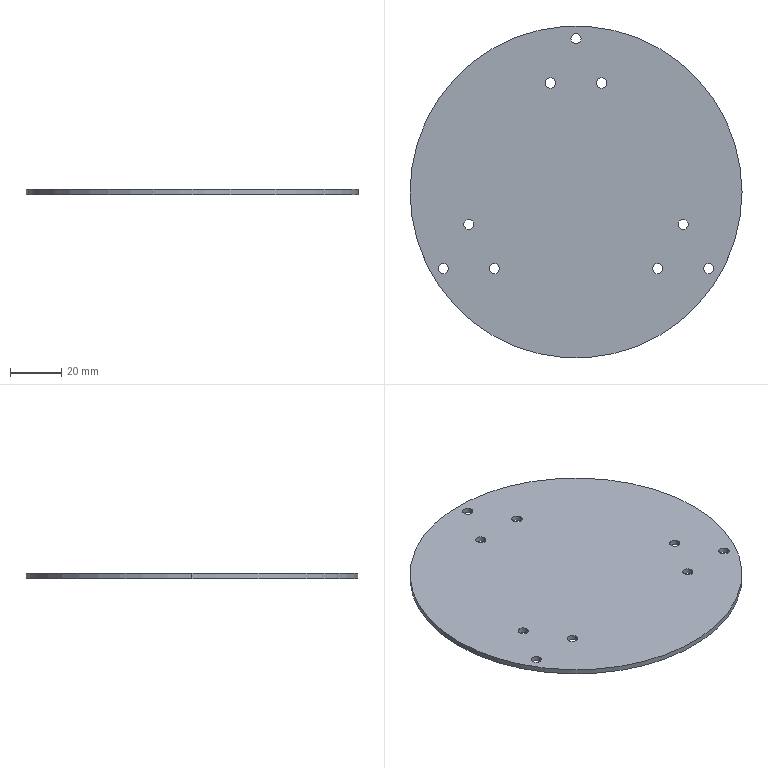Part | SolidWorks | features Extrusion 1, ICE 1 | 1 solid | 22 faces | box 130 x 130 x 2 mm | volume 26320 mm3 | cylinder 20 | plane 2 | commonest cylinder face diameters 4 x18 130 x2
STEP:
#1=CARTESIAN_POINT('',(-33.962,-30.,0.));
#2=VERTEX_POINT('',#1);
#3=CARTESIAN_POINT('',(-29.962,-30.,0.));
#4=VERTEX_POINT('',#3);
#5=CARTESIAN_POINT('',(-31.962,-30.,0.));
#6=DIRECTION('',(0.,0.,1.));
#7=DIRECTION('',(1.,0.,0.));
#8=AXIS2_PLACEMENT_3D('',#5,#6,#7);
#9=CIRCLE('',#8,2.);
#10=EDGE_CURVE('',#2,#4,#9,.T.);
#11=ORIENTED_EDGE('',*,*,#10,.F.);
#12=CARTESIAN_POINT('',(-33.962,-30.,2.));
#13=VERTEX_POINT('',#12);
#14=CARTESIAN_POINT('',(-33.962,-30.,0.));
#15=DIRECTION('',(0.,0.,1.));
#16=VECTOR('',#15,1000.);
#17=LINE('',#14,#16);
#18=EDGE_CURVE('',#2,#13,#17,.T.);
#19=ORIENTED_EDGE('',*,*,#18,.T.);
#20=CARTESIAN_POINT('',(-29.962,-30.,2.));
#21=VERTEX_POINT('',#20);
#22=CARTESIAN_POINT('',(-31.962,-30.,2.));
#23=DIRECTION('',(0.,0.,1.));
#24=DIRECTION('',(1.,0.,0.));
#25=AXIS2_PLACEMENT_3D('',#22,#23,#24);
#26=CIRCLE('',#25,2.);
#27=EDGE_CURVE('',#13,#21,#26,.T.);
#28=ORIENTED_EDGE('',*,*,#27,.T.);
#29=CARTESIAN_POINT('',(-29.962,-30.,0.));
#30=DIRECTION('',(0.,0.,1.));
#31=VECTOR('',#30,1000.);
#32=LINE('',#29,#31);
#33=EDGE_CURVE('',#4,#21,#32,.T.);
#34=ORIENTED_EDGE('',*,*,#33,.F.);
#35=EDGE_LOOP('',(#11,#19,#28,#34));
#36=FACE_OUTER_BOUND('',#35,.T.);
#37=CARTESIAN_POINT('',(-31.962,-30.,0.));
#38=DIRECTION('',(0.,0.,1.));
#39=DIRECTION('',(1.,0.,0.));
#40=AXIS2_PLACEMENT_3D('',#37,#38,#39);
#41=CYLINDRICAL_SURFACE('',#40,2.);
#42=ADVANCED_FACE('',(#36),#41,.F.);
#43=CARTESIAN_POINT('',(-43.962,-12.679,0.));
#44=VERTEX_POINT('',#43);
#45=CARTESIAN_POINT('',(-39.962,-12.679,0.));
#46=VERTEX_POINT('',#45);
#47=CARTESIAN_POINT('',(-41.962,-12.679,0.));
#48=DIRECTION('',(0.,0.,1.));
#49=DIRECTION('',(1.,0.,0.));
#50=AXIS2_PLACEMENT_3D('',#47,#48,#49);
#51=CIRCLE('',#50,2.);
#52=EDGE_CURVE('',#44,#46,#51,.T.);
#53=ORIENTED_EDGE('',*,*,#52,.F.);
#54=CARTESIAN_POINT('',(-43.962,-12.679,2.));
#55=VERTEX_POINT('',#54);
#56=CARTESIAN_POINT('',(-43.962,-12.679,0.));
#57=DIRECTION('',(0.,0.,1.));
#58=VECTOR('',#57,1000.);
#59=LINE('',#56,#58);
#60=EDGE_CURVE('',#44,#55,#59,.T.);
#61=ORIENTED_EDGE('',*,*,#60,.T.);
#62=CARTESIAN_POINT('',(-39.962,-12.679,2.));
#63=VERTEX_POINT('',#62);
#64=CARTESIAN_POINT('',(-41.962,-12.679,2.));
#65=DIRECTION('',(0.,0.,1.));
#66=DIRECTION('',(1.,0.,0.));
#67=AXIS2_PLACEMENT_3D('',#64,#65,#66);
#68=CIRCLE('',#67,2.);
#69=EDGE_CURVE('',#55,#63,#68,.T.);
#70=ORIENTED_EDGE('',*,*,#69,.T.);
#71=CARTESIAN_POINT('',(-39.962,-12.679,0.));
#72=DIRECTION('',(0.,0.,1.));
#73=VECTOR('',#72,1000.);
#74=LINE('',#71,#73);
#75=EDGE_CURVE('',#46,#63,#74,.T.);
#76=ORIENTED_EDGE('',*,*,#75,.F.);
#77=EDGE_LOOP('',(#53,#61,#70,#76));
#78=FACE_OUTER_BOUND('',#77,.T.);
#79=CARTESIAN_POINT('',(-41.962,-12.679,0.));
#80=DIRECTION('',(0.,0.,1.));
#81=DIRECTION('',(1.,0.,0.));
#82=AXIS2_PLACEMENT_3D('',#79,#80,#81);
#83=CYLINDRICAL_SURFACE('',#82,2.);
#84=ADVANCED_FACE('',(#78),#83,.F.);
#85=CARTESIAN_POINT('',(-53.962,-30.,0.));
#86=VERTEX_POINT('',#85);
#87=CARTESIAN_POINT('',(-49.962,-30.,0.));
#88=VERTEX_POINT('',#87);
#89=CARTESIAN_POINT('',(-51.962,-30.,0.));
#90=DIRECTION('',(0.,0.,1.));
#91=DIRECTION('',(1.,0.,0.));
#92=AXIS2_PLACEMENT_3D('',#89,#90,#91);
#93=CIRCLE('',#92,2.);
#94=EDGE_CURVE('',#86,#88,#93,.T.);
#95=ORIENTED_EDGE('',*,*,#94,.F.);
#96=CARTESIAN_POINT('',(-53.962,-30.,2.));
#97=VERTEX_POINT('',#96);
#98=CARTESIAN_POINT('',(-53.962,-30.,0.));
#99=DIRECTION('',(0.,0.,1.));
#100=VECTOR('',#99,1000.);
#101=LINE('',#98,#100);
#102=EDGE_CURVE('',#86,#97,#101,.T.);
#103=ORIENTED_EDGE('',*,*,#102,.T.);
#104=CARTESIAN_POINT('',(-49.962,-30.,2.));
#105=VERTEX_POINT('',#104);
#106=CARTESIAN_POINT('',(-51.962,-30.,2.));
#107=DIRECTION('',(0.,0.,1.));
#108=DIRECTION('',(1.,0.,0.));
#109=AXIS2_PLACEMENT_3D('',#106,#107,#108);
#110=CIRCLE('',#109,2.);
#111=EDGE_CURVE('',#97,#105,#110,.T.);
#112=ORIENTED_EDGE('',*,*,#111,.T.);
#113=CARTESIAN_POINT('',(-49.962,-30.,0.));
#114=DIRECTION('',(0.,0.,1.));
#115=VECTOR('',#114,1000.);
#116=LINE('',#113,#115);
#117=EDGE_CURVE('',#88,#105,#116,.T.);
#118=ORIENTED_EDGE('',*,*,#117,.F.);
#119=EDGE_LOOP('',(#95,#103,#112,#118));
#120=FACE_OUTER_BOUND('',#119,.T.);
#121=CARTESIAN_POINT('',(-51.962,-30.,0.));
#122=DIRECTION('',(0.,0.,1.));
#123=DIRECTION('',(1.,0.,0.));
#124=AXIS2_PLACEMENT_3D('',#121,#122,#123);
#125=CYLINDRICAL_SURFACE('',#124,2.);
#126=ADVANCED_FACE('',(#120),#125,.F.);
#127=CARTESIAN_POINT('',(39.962,-12.679,0.));
#128=VERTEX_POINT('',#127);
#129=CARTESIAN_POINT('',(43.962,-12.679,0.));
#130=VERTEX_POINT('',#129);
#131=CARTESIAN_POINT('',(41.962,-12.679,0.));
#132=DIRECTION('',(0.,0.,1.));
#133=DIRECTION('',(1.,0.,0.));
#134=AXIS2_PLACEMENT_3D('',#131,#132,#133);
#135=CIRCLE('',#134,2.);
#136=EDGE_CURVE('',#128,#130,#135,.T.);
#137=ORIENTED_EDGE('',*,*,#136,.F.);
#138=CARTESIAN_POINT('',(39.962,-12.679,2.));
#139=VERTEX_POINT('',#138);
#140=CARTESIAN_POINT('',(39.962,-12.679,0.));
#141=DIRECTION('',(0.,0.,1.));
#142=VECTOR('',#141,1000.);
#143=LINE('',#140,#142);
#144=EDGE_CURVE('',#128,#139,#143,.T.);
#145=ORIENTED_EDGE('',*,*,#144,.T.);
#146=CARTESIAN_POINT('',(43.962,-12.679,2.));
#147=VERTEX_POINT('',#146);
#148=CARTESIAN_POINT('',(41.962,-12.679,2.));
#149=DIRECTION('',(0.,0.,1.));
#150=DIRECTION('',(1.,0.,0.));
#151=AXIS2_PLACEMENT_3D('',#148,#149,#150);
#152=CIRCLE('',#151,2.);
#153=EDGE_CURVE('',#139,#147,#152,.T.);
#154=ORIENTED_EDGE('',*,*,#153,.T.);
#155=CARTESIAN_POINT('',(43.962,-12.679,0.));
#156=DIRECTION('',(0.,0.,1.));
#157=VECTOR('',#156,1000.);
#158=LINE('',#155,#157);
#159=EDGE_CURVE('',#130,#147,#158,.T.);
#160=ORIENTED_EDGE('',*,*,#159,.F.);
#161=EDGE_LOOP('',(#137,#145,#154,#160));
#162=FACE_OUTER_BOUND('',#161,.T.);
#163=CARTESIAN_POINT('',(41.962,-12.679,0.));
#164=DIRECTION('',(0.,0.,1.));
#165=DIRECTION('',(1.,0.,0.));
#166=AXIS2_PLACEMENT_3D('',#163,#164,#165);
#167=CYLINDRICAL_SURFACE('',#166,2.);
#168=ADVANCED_FACE('',(#162),#167,.F.);
#169=CARTESIAN_POINT('',(29.962,-30.,0.));
#170=VERTEX_POINT('',#169);
#171=CARTESIAN_POINT('',(33.962,-30.,0.));
#172=VERTEX_POINT('',#171);
#173=CARTESIAN_POINT('',(31.962,-30.,0.));
#174=DIRECTION('',(0.,0.,1.));
#175=DIRECTION('',(1.,0.,0.));
#176=AXIS2_PLACEMENT_3D('',#173,#174,#175);
#177=CIRCLE('',#176,2.);
#178=EDGE_CURVE('',#170,#172,#177,.T.);
#179=ORIENTED_EDGE('',*,*,#178,.F.);
#180=CARTESIAN_POINT('',(29.962,-30.,2.));
#181=VERTEX_POINT('',#180);
#182=CARTESIAN_POINT('',(29.962,-30.,0.));
#183=DIRECTION('',(0.,0.,1.));
#184=VECTOR('',#183,1000.);
#185=LINE('',#182,#184);
#186=EDGE_CURVE('',#170,#181,#185,.T.);
#187=ORIENTED_EDGE('',*,*,#186,.T.);
#188=CARTESIAN_POINT('',(33.962,-30.,2.));
#189=VERTEX_POINT('',#188);
#190=CARTESIAN_POINT('',(31.962,-30.,2.));
#191=DIRECTION('',(0.,0.,1.));
#192=DIRECTION('',(1.,0.,0.));
#193=AXIS2_PLACEMENT_3D('',#190,#191,#192);
#194=CIRCLE('',#193,2.);
#195=EDGE_CURVE('',#181,#189,#194,.T.);
#196=ORIENTED_EDGE('',*,*,#195,.T.);
#197=CARTESIAN_POINT('',(33.962,-30.,0.));
#198=DIRECTION('',(0.,0.,1.));
#199=VECTOR('',#198,1000.);
#200=LINE('',#197,#199);
#201=EDGE_CURVE('',#172,#189,#200,.T.);
#202=ORIENTED_EDGE('',*,*,#201,.F.);
#203=EDGE_LOOP('',(#179,#187,#196,#202));
#204=FACE_OUTER_BOUND('',#203,.T.);
#205=CARTESIAN_POINT('',(31.962,-30.,0.));
#206=DIRECTION('',(0.,0.,1.));
#207=DIRECTION('',(1.,0.,0.));
#208=AXIS2_PLACEMENT_3D('',#205,#206,#207);
#209=CYLINDRICAL_SURFACE('',#208,2.);
#210=ADVANCED_FACE('',(#204),#209,.F.);
#211=CARTESIAN_POINT('',(49.962,-30.,0.));
#212=VERTEX_POINT('',#211);
#213=CARTESIAN_POINT('',(53.962,-30.,0.));
#214=VERTEX_POINT('',#213);
#215=CARTESIAN_POINT('',(51.962,-30.,0.));
#216=DIRECTION('',(0.,0.,1.));
#217=DIRECTION('',(1.,0.,0.));
#218=AXIS2_PLACEMENT_3D('',#215,#216,#217);
#219=CIRCLE('',#218,2.);
#220=EDGE_CURVE('',#212,#214,#219,.T.);
#221=ORIENTED_EDGE('',*,*,#220,.F.);
#222=CARTESIAN_POINT('',(49.962,-30.,2.));
#223=VERTEX_POINT('',#222);
#224=CARTESIAN_POINT('',(49.962,-30.,0.));
#225=DIRECTION('',(0.,0.,1.));
#226=VECTOR('',#225,1000.);
#227=LINE('',#224,#226);
#228=EDGE_CURVE('',#212,#223,#227,.T.);
#229=ORIENTED_EDGE('',*,*,#228,.T.);
#230=CARTESIAN_POINT('',(53.962,-30.,2.));
#231=VERTEX_POINT('',#230);
#232=CARTESIAN_POINT('',(51.962,-30.,2.));
#233=DIRECTION('',(0.,0.,1.));
#234=DIRECTION('',(1.,0.,0.));
#235=AXIS2_PLACEMENT_3D('',#232,#233,#234);
#236=CIRCLE('',#235,2.);
#237=EDGE_CURVE('',#223,#231,#236,.T.);
#238=ORIENTED_EDGE('',*,*,#237,.T.);
#239=CARTESIAN_POINT('',(53.962,-30.,0.));
#240=DIRECTION('',(0.,0.,1.));
#241=VECTOR('',#240,1000.);
#242=LINE('',#239,#241);
#243=EDGE_CURVE('',#214,#231,#242,.T.);
#244=ORIENTED_EDGE('',*,*,#243,.F.);
#245=EDGE_LOOP('',(#221,#229,#238,#244));
#246=FACE_OUTER_BOUND('',#245,.T.);
#247=CARTESIAN_POINT('',(51.962,-30.,0.));
#248=DIRECTION('',(0.,0.,1.));
#249=DIRECTION('',(1.,0.,0.));
#250=AXIS2_PLACEMENT_3D('',#247,#248,#249);
#251=CYLINDRICAL_SURFACE('',#250,2.);
#252=ADVANCED_FACE('',(#246),#251,.F.);
#253=CARTESIAN_POINT('',(-12.,42.679,0.));
#254=VERTEX_POINT('',#253);
#255=CARTESIAN_POINT('',(-8.,42.679,0.));
#256=VERTEX_POINT('',#255);
#257=CARTESIAN_POINT('',(-10.,42.679,0.));
#258=DIRECTION('',(0.,0.,1.));
#259=DIRECTION('',(1.,0.,0.));
#260=AXIS2_PLACEMENT_3D('',#257,#258,#259);
#261=CIRCLE('',#260,2.);
#262=EDGE_CURVE('',#254,#256,#261,.T.);
#263=ORIENTED_EDGE('',*,*,#262,.F.);
#264=CARTESIAN_POINT('',(-12.,42.679,2.));
#265=VERTEX_POINT('',#264);
#266=CARTESIAN_POINT('',(-12.,42.679,0.));
#267=DIRECTION('',(0.,0.,1.));
#268=VECTOR('',#267,1000.);
#269=LINE('',#266,#268);
#270=EDGE_CURVE('',#254,#265,#269,.T.);
#271=ORIENTED_EDGE('',*,*,#270,.T.);
#272=CARTESIAN_POINT('',(-8.,42.679,2.));
#273=VERTEX_POINT('',#272);
#274=CARTESIAN_POINT('',(-10.,42.679,2.));
#275=DIRECTION('',(0.,0.,1.));
#276=DIRECTION('',(1.,0.,0.));
#277=AXIS2_PLACEMENT_3D('',#274,#275,#276);
#278=CIRCLE('',#277,2.);
#279=EDGE_CURVE('',#265,#273,#278,.T.);
#280=ORIENTED_EDGE('',*,*,#279,.T.);
#281=CARTESIAN_POINT('',(-8.,42.679,0.));
#282=DIRECTION('',(0.,0.,1.));
#283=VECTOR('',#282,1000.);
#284=LINE('',#281,#283);
#285=EDGE_CURVE('',#256,#273,#284,.T.);
#286=ORIENTED_EDGE('',*,*,#285,.F.);
#287=EDGE_LOOP('',(#263,#271,#280,#286));
#288=FACE_OUTER_BOUND('',#287,.T.);
#289=CARTESIAN_POINT('',(-10.,42.679,0.));
#290=DIRECTION('',(0.,0.,1.));
#291=DIRECTION('',(1.,0.,0.));
#292=AXIS2_PLACEMENT_3D('',#289,#290,#291);
#293=CYLINDRICAL_SURFACE('',#292,2.);
#294=ADVANCED_FACE('',(#288),#293,.F.);
#295=CARTESIAN_POINT('',(8.,42.679,0.));
#296=VERTEX_POINT('',#295);
#297=CARTESIAN_POINT('',(12.,42.679,0.));
#298=VERTEX_POINT('',#297);
#299=CARTESIAN_POINT('',(10.,42.679,0.));
#300=DIRECTION('',(0.,0.,1.));
#301=DIRECTION('',(1.,0.,0.));
#302=AXIS2_PLACEMENT_3D('',#299,#300,#301);
#303=CIRCLE('',#302,2.);
#304=EDGE_CURVE('',#296,#298,#303,.T.);
#305=ORIENTED_EDGE('',*,*,#304,.F.);
#306=CARTESIAN_POINT('',(8.,42.679,2.));
#307=VERTEX_POINT('',#306);
#308=CARTESIAN_POINT('',(8.,42.679,0.));
#309=DIRECTION('',(0.,0.,1.));
#310=VECTOR('',#309,1000.);
#311=LINE('',#308,#310);
#312=EDGE_CURVE('',#296,#307,#311,.T.);
#313=ORIENTED_EDGE('',*,*,#312,.T.);
#314=CARTESIAN_POINT('',(12.,42.679,2.));
#315=VERTEX_POINT('',#314);
#316=CARTESIAN_POINT('',(10.,42.679,2.));
#317=DIRECTION('',(0.,0.,1.));
#318=DIRECTION('',(1.,0.,0.));
#319=AXIS2_PLACEMENT_3D('',#316,#317,#318);
#320=CIRCLE('',#319,2.);
#321=EDGE_CURVE('',#307,#315,#320,.T.);
#322=ORIENTED_EDGE('',*,*,#321,.T.);
#323=CARTESIAN_POINT('',(12.,42.679,0.));
#324=DIRECTION('',(0.,0.,1.));
#325=VECTOR('',#324,1000.);
#326=LINE('',#323,#325);
#327=EDGE_CURVE('',#298,#315,#326,.T.);
#328=ORIENTED_EDGE('',*,*,#327,.F.);
#329=EDGE_LOOP('',(#305,#313,#322,#328));
#330=FACE_OUTER_BOUND('',#329,.T.);
#331=CARTESIAN_POINT('',(10.,42.679,0.));
#332=DIRECTION('',(0.,0.,1.));
#333=DIRECTION('',(1.,0.,0.));
#334=AXIS2_PLACEMENT_3D('',#331,#332,#333);
#335=CYLINDRICAL_SURFACE('',#334,2.);
#336=ADVANCED_FACE('',(#330),#335,.F.);
#337=CARTESIAN_POINT('',(-2.,60.,0.));
#338=VERTEX_POINT('',#337);
#339=CARTESIAN_POINT('',(2.,60.,0.));
#340=VERTEX_POINT('',#339);
#341=CARTESIAN_POINT('',(0.,60.,0.));
#342=DIRECTION('',(0.,0.,1.));
#343=DIRECTION('',(1.,0.,0.));
#344=AXIS2_PLACEMENT_3D('',#341,#342,#343);
#345=CIRCLE('',#344,2.);
#346=EDGE_CURVE('',#338,#340,#345,.T.);
#347=ORIENTED_EDGE('',*,*,#346,.F.);
#348=CARTESIAN_POINT('',(-2.,60.,2.));
#349=VERTEX_POINT('',#348);
#350=CARTESIAN_POINT('',(-2.,60.,0.));
#351=DIRECTION('',(0.,0.,1.));
#352=VECTOR('',#351,1000.);
#353=LINE('',#350,#352);
#354=EDGE_CURVE('',#338,#349,#353,.T.);
#355=ORIENTED_EDGE('',*,*,#354,.T.);
#356=CARTESIAN_POINT('',(2.,60.,2.));
#357=VERTEX_POINT('',#356);
#358=CARTESIAN_POINT('',(0.,60.,2.));
#359=DIRECTION('',(0.,0.,1.));
#360=DIRECTION('',(1.,0.,0.));
#361=AXIS2_PLACEMENT_3D('',#358,#359,#360);
#362=CIRCLE('',#361,2.);
#363=EDGE_CURVE('',#349,#357,#362,.T.);
#364=ORIENTED_EDGE('',*,*,#363,.T.);
#365=CARTESIAN_POINT('',(2.,60.,0.));
#366=DIRECTION('',(0.,0.,1.));
#367=VECTOR('',#366,1000.);
#368=LINE('',#365,#367);
#369=EDGE_CURVE('',#340,#357,#368,.T.);
#370=ORIENTED_EDGE('',*,*,#369,.F.);
#371=EDGE_LOOP('',(#347,#355,#364,#370));
#372=FACE_OUTER_BOUND('',#371,.T.);
#373=CARTESIAN_POINT('',(0.,60.,0.));
#374=DIRECTION('',(0.,0.,1.));
#375=DIRECTION('',(1.,0.,0.));
#376=AXIS2_PLACEMENT_3D('',#373,#374,#375);
#377=CYLINDRICAL_SURFACE('',#376,2.);
#378=ADVANCED_FACE('',(#372),#377,.F.);
#379=CARTESIAN_POINT('',(65.,0.,2.));
#380=VERTEX_POINT('',#379);
#381=CARTESIAN_POINT('',(-65.,0.,2.));
#382=VERTEX_POINT('',#381);
#383=CARTESIAN_POINT('',(0.,0.,2.));
#384=DIRECTION('',(0.,0.,1.));
#385=DIRECTION('',(1.,0.,0.));
#386=AXIS2_PLACEMENT_3D('',#383,#384,#385);
#387=CIRCLE('',#386,65.);
#388=EDGE_CURVE('',#380,#382,#387,.T.);
#389=ORIENTED_EDGE('',*,*,#388,.F.);
#390=CARTESIAN_POINT('',(65.,0.,0.));
#391=VERTEX_POINT('',#390);
#392=CARTESIAN_POINT('',(65.,0.,2.));
#393=DIRECTION('',(0.,0.,-1.));
#394=VECTOR('',#393,1000.);
#395=LINE('',#392,#394);
#396=EDGE_CURVE('',#380,#391,#395,.T.);
#397=ORIENTED_EDGE('',*,*,#396,.T.);
#398=CARTESIAN_POINT('',(-65.,0.,0.));
#399=VERTEX_POINT('',#398);
#400=CARTESIAN_POINT('',(0.,0.,0.));
#401=DIRECTION('',(0.,0.,1.));
#402=DIRECTION('',(1.,0.,0.));
#403=AXIS2_PLACEMENT_3D('',#400,#401,#402);
#404=CIRCLE('',#403,65.);
#405=EDGE_CURVE('',#391,#399,#404,.T.);
#406=ORIENTED_EDGE('',*,*,#405,.T.);
#407=CARTESIAN_POINT('',(-65.,0.,2.));
#408=DIRECTION('',(0.,0.,-1.));
#409=VECTOR('',#408,1000.);
#410=LINE('',#407,#409);
#411=EDGE_CURVE('',#382,#399,#410,.T.);
#412=ORIENTED_EDGE('',*,*,#411,.F.);
#413=EDGE_LOOP('',(#389,#397,#406,#412));
#414=FACE_OUTER_BOUND('',#413,.T.);
#415=CARTESIAN_POINT('',(0.,0.,2.));
#416=DIRECTION('',(0.,0.,-1.));
#417=DIRECTION('',(-1.,0.,0.));
#418=AXIS2_PLACEMENT_3D('',#415,#416,#417);
#419=CYLINDRICAL_SURFACE('',#418,65.);
#420=ADVANCED_FACE('',(#414),#419,.T.);
#421=ORIENTED_EDGE('',*,*,#396,.F.);
#422=CARTESIAN_POINT('',(0.,0.,2.));
#423=DIRECTION('',(0.,0.,1.));
#424=DIRECTION('',(1.,0.,0.));
#425=AXIS2_PLACEMENT_3D('',#422,#423,#424);
#426=CIRCLE('',#425,65.);
#427=EDGE_CURVE('',#382,#380,#426,.T.);
#428=ORIENTED_EDGE('',*,*,#427,.F.);
#429=ORIENTED_EDGE('',*,*,#411,.T.);
#430=CARTESIAN_POINT('',(0.,0.,0.));
#431=DIRECTION('',(0.,0.,1.));
#432=DIRECTION('',(1.,0.,0.));
#433=AXIS2_PLACEMENT_3D('',#430,#431,#432);
#434=CIRCLE('',#433,65.);
#435=EDGE_CURVE('',#399,#391,#434,.T.);
#436=ORIENTED_EDGE('',*,*,#435,.T.);
#437=EDGE_LOOP('',(#421,#428,#429,#436));
#438=FACE_OUTER_BOUND('',#437,.T.);
#439=CARTESIAN_POINT('',(0.,0.,2.));
#440=DIRECTION('',(0.,0.,-1.));
#441=DIRECTION('',(-1.,0.,0.));
#442=AXIS2_PLACEMENT_3D('',#439,#440,#441);
#443=CYLINDRICAL_SURFACE('',#442,65.);
#444=ADVANCED_FACE('',(#438),#443,.T.);
#445=CARTESIAN_POINT('',(-31.962,-30.,2.));
#446=DIRECTION('',(0.,0.,1.));
#447=DIRECTION('',(1.,0.,0.));
#448=AXIS2_PLACEMENT_3D('',#445,#446,#447);
#449=CIRCLE('',#448,2.);
#450=EDGE_CURVE('',#21,#13,#449,.T.);
#451=ORIENTED_EDGE('',*,*,#450,.F.);
#452=ORIENTED_EDGE('',*,*,#27,.F.);
#453=EDGE_LOOP('',(#451,#452));
#454=FACE_BOUND('',#453,.T.);
#455=CARTESIAN_POINT('',(-41.962,-12.679,2.));
#456=DIRECTION('',(0.,0.,1.));
#457=DIRECTION('',(1.,0.,0.));
#458=AXIS2_PLACEMENT_3D('',#455,#456,#457);
#459=CIRCLE('',#458,2.);
#460=EDGE_CURVE('',#63,#55,#459,.T.);
#461=ORIENTED_EDGE('',*,*,#460,.F.);
#462=ORIENTED_EDGE('',*,*,#69,.F.);
#463=EDGE_LOOP('',(#461,#462));
#464=FACE_BOUND('',#463,.T.);
#465=CARTESIAN_POINT('',(-51.962,-30.,2.));
#466=DIRECTION('',(0.,0.,1.));
#467=DIRECTION('',(1.,0.,0.));
#468=AXIS2_PLACEMENT_3D('',#465,#466,#467);
#469=CIRCLE('',#468,2.);
#470=EDGE_CURVE('',#105,#97,#469,.T.);
#471=ORIENTED_EDGE('',*,*,#470,.F.);
#472=ORIENTED_EDGE('',*,*,#111,.F.);
#473=EDGE_LOOP('',(#471,#472));
#474=FACE_BOUND('',#473,.T.);
#475=CARTESIAN_POINT('',(41.962,-12.679,2.));
#476=DIRECTION('',(0.,0.,1.));
#477=DIRECTION('',(1.,0.,0.));
#478=AXIS2_PLACEMENT_3D('',#475,#476,#477);
#479=CIRCLE('',#478,2.);
#480=EDGE_CURVE('',#147,#139,#479,.T.);
#481=ORIENTED_EDGE('',*,*,#480,.F.);
#482=ORIENTED_EDGE('',*,*,#153,.F.);
#483=EDGE_LOOP('',(#481,#482));
#484=FACE_BOUND('',#483,.T.);
#485=CARTESIAN_POINT('',(31.962,-30.,2.));
#486=DIRECTION('',(0.,0.,1.));
#487=DIRECTION('',(1.,0.,0.));
#488=AXIS2_PLACEMENT_3D('',#485,#486,#487);
#489=CIRCLE('',#488,2.);
#490=EDGE_CURVE('',#189,#181,#489,.T.);
#491=ORIENTED_EDGE('',*,*,#490,.F.);
#492=ORIENTED_EDGE('',*,*,#195,.F.);
#493=EDGE_LOOP('',(#491,#492));
#494=FACE_BOUND('',#493,.T.);
#495=CARTESIAN_POINT('',(51.962,-30.,2.));
#496=DIRECTION('',(0.,0.,1.));
#497=DIRECTION('',(1.,0.,0.));
#498=AXIS2_PLACEMENT_3D('',#495,#496,#497);
#499=CIRCLE('',#498,2.);
#500=EDGE_CURVE('',#231,#223,#499,.T.);
#501=ORIENTED_EDGE('',*,*,#500,.F.);
#502=ORIENTED_EDGE('',*,*,#237,.F.);
#503=EDGE_LOOP('',(#501,#502));
#504=FACE_BOUND('',#503,.T.);
#505=CARTESIAN_POINT('',(-10.,42.679,2.));
#506=DIRECTION('',(0.,0.,1.));
#507=DIRECTION('',(1.,0.,0.));
#508=AXIS2_PLACEMENT_3D('',#505,#506,#507);
#509=CIRCLE('',#508,2.);
#510=EDGE_CURVE('',#273,#265,#509,.T.);
#511=ORIENTED_EDGE('',*,*,#510,.F.);
#512=ORIENTED_EDGE('',*,*,#279,.F.);
#513=EDGE_LOOP('',(#511,#512));
#514=FACE_BOUND('',#513,.T.);
#515=CARTESIAN_POINT('',(10.,42.679,2.));
#516=DIRECTION('',(0.,0.,1.));
#517=DIRECTION('',(1.,0.,0.));
#518=AXIS2_PLACEMENT_3D('',#515,#516,#517);
#519=CIRCLE('',#518,2.);
#520=EDGE_CURVE('',#315,#307,#519,.T.);
#521=ORIENTED_EDGE('',*,*,#520,.F.);
#522=ORIENTED_EDGE('',*,*,#321,.F.);
#523=EDGE_LOOP('',(#521,#522));
#524=FACE_BOUND('',#523,.T.);
#525=CARTESIAN_POINT('',(0.,60.,2.));
#526=DIRECTION('',(0.,0.,1.));
#527=DIRECTION('',(1.,0.,0.));
#528=AXIS2_PLACEMENT_3D('',#525,#526,#527);
#529=CIRCLE('',#528,2.);
#530=EDGE_CURVE('',#357,#349,#529,.T.);
#531=ORIENTED_EDGE('',*,*,#530,.F.);
#532=ORIENTED_EDGE('',*,*,#363,.F.);
#533=EDGE_LOOP('',(#531,#532));
#534=FACE_BOUND('',#533,.T.);
#535=ORIENTED_EDGE('',*,*,#427,.T.);
#536=ORIENTED_EDGE('',*,*,#388,.T.);
#537=EDGE_LOOP('',(#535,#536));
#538=FACE_OUTER_BOUND('',#537,.T.);
#539=CARTESIAN_POINT('',(0.,0.,2.));
#540=DIRECTION('',(0.,0.,1.));
#541=DIRECTION('',(1.,0.,0.));
#542=AXIS2_PLACEMENT_3D('',#539,#540,#541);
#543=PLANE('',#542);
#544=ADVANCED_FACE('',(#454,#464,#474,#484,#494,#504,#514,#524,#534,#538),#543,.T.);
#545=CARTESIAN_POINT('',(-31.962,-30.,0.));
#546=DIRECTION('',(0.,0.,1.));
#547=DIRECTION('',(1.,0.,0.));
#548=AXIS2_PLACEMENT_3D('',#545,#546,#547);
#549=CIRCLE('',#548,2.);
#550=EDGE_CURVE('',#4,#2,#549,.T.);
#551=ORIENTED_EDGE('',*,*,#550,.T.);
#552=ORIENTED_EDGE('',*,*,#10,.T.);
#553=EDGE_LOOP('',(#551,#552));
#554=FACE_BOUND('',#553,.T.);
#555=CARTESIAN_POINT('',(-41.962,-12.679,0.));
#556=DIRECTION('',(0.,0.,1.));
#557=DIRECTION('',(1.,0.,0.));
#558=AXIS2_PLACEMENT_3D('',#555,#556,#557);
#559=CIRCLE('',#558,2.);
#560=EDGE_CURVE('',#46,#44,#559,.T.);
#561=ORIENTED_EDGE('',*,*,#560,.T.);
#562=ORIENTED_EDGE('',*,*,#52,.T.);
#563=EDGE_LOOP('',(#561,#562));
#564=FACE_BOUND('',#563,.T.);
#565=CARTESIAN_POINT('',(-51.962,-30.,0.));
#566=DIRECTION('',(0.,0.,1.));
#567=DIRECTION('',(1.,0.,0.));
#568=AXIS2_PLACEMENT_3D('',#565,#566,#567);
#569=CIRCLE('',#568,2.);
#570=EDGE_CURVE('',#88,#86,#569,.T.);
#571=ORIENTED_EDGE('',*,*,#570,.T.);
#572=ORIENTED_EDGE('',*,*,#94,.T.);
#573=EDGE_LOOP('',(#571,#572));
#574=FACE_BOUND('',#573,.T.);
#575=CARTESIAN_POINT('',(41.962,-12.679,0.));
#576=DIRECTION('',(0.,0.,1.));
#577=DIRECTION('',(1.,0.,0.));
#578=AXIS2_PLACEMENT_3D('',#575,#576,#577);
#579=CIRCLE('',#578,2.);
#580=EDGE_CURVE('',#130,#128,#579,.T.);
#581=ORIENTED_EDGE('',*,*,#580,.T.);
#582=ORIENTED_EDGE('',*,*,#136,.T.);
#583=EDGE_LOOP('',(#581,#582));
#584=FACE_BOUND('',#583,.T.);
#585=CARTESIAN_POINT('',(31.962,-30.,0.));
#586=DIRECTION('',(0.,0.,1.));
#587=DIRECTION('',(1.,0.,0.));
#588=AXIS2_PLACEMENT_3D('',#585,#586,#587);
#589=CIRCLE('',#588,2.);
#590=EDGE_CURVE('',#172,#170,#589,.T.);
#591=ORIENTED_EDGE('',*,*,#590,.T.);
#592=ORIENTED_EDGE('',*,*,#178,.T.);
#593=EDGE_LOOP('',(#591,#592));
#594=FACE_BOUND('',#593,.T.);
#595=CARTESIAN_POINT('',(51.962,-30.,0.));
#596=DIRECTION('',(0.,0.,1.));
#597=DIRECTION('',(1.,0.,0.));
#598=AXIS2_PLACEMENT_3D('',#595,#596,#597);
#599=CIRCLE('',#598,2.);
#600=EDGE_CURVE('',#214,#212,#599,.T.);
#601=ORIENTED_EDGE('',*,*,#600,.T.);
#602=ORIENTED_EDGE('',*,*,#220,.T.);
#603=EDGE_LOOP('',(#601,#602));
#604=FACE_BOUND('',#603,.T.);
#605=CARTESIAN_POINT('',(-10.,42.679,0.));
#606=DIRECTION('',(0.,0.,1.));
#607=DIRECTION('',(1.,0.,0.));
#608=AXIS2_PLACEMENT_3D('',#605,#606,#607);
#609=CIRCLE('',#608,2.);
#610=EDGE_CURVE('',#256,#254,#609,.T.);
#611=ORIENTED_EDGE('',*,*,#610,.T.);
#612=ORIENTED_EDGE('',*,*,#262,.T.);
#613=EDGE_LOOP('',(#611,#612));
#614=FACE_BOUND('',#613,.T.);
#615=CARTESIAN_POINT('',(10.,42.679,0.));
#616=DIRECTION('',(0.,0.,1.));
#617=DIRECTION('',(1.,0.,0.));
#618=AXIS2_PLACEMENT_3D('',#615,#616,#617);
#619=CIRCLE('',#618,2.);
#620=EDGE_CURVE('',#298,#296,#619,.T.);
#621=ORIENTED_EDGE('',*,*,#620,.T.);
#622=ORIENTED_EDGE('',*,*,#304,.T.);
#623=EDGE_LOOP('',(#621,#622));
#624=FACE_BOUND('',#623,.T.);
#625=CARTESIAN_POINT('',(0.,60.,0.));
#626=DIRECTION('',(0.,0.,1.));
#627=DIRECTION('',(1.,0.,0.));
#628=AXIS2_PLACEMENT_3D('',#625,#626,#627);
#629=CIRCLE('',#628,2.);
#630=EDGE_CURVE('',#340,#338,#629,.T.);
#631=ORIENTED_EDGE('',*,*,#630,.T.);
#632=ORIENTED_EDGE('',*,*,#346,.T.);
#633=EDGE_LOOP('',(#631,#632));
#634=FACE_BOUND('',#633,.T.);
#635=ORIENTED_EDGE('',*,*,#435,.F.);
#636=ORIENTED_EDGE('',*,*,#405,.F.);
#637=EDGE_LOOP('',(#635,#636));
#638=FACE_OUTER_BOUND('',#637,.T.);
#639=CARTESIAN_POINT('',(0.,0.,0.));
#640=DIRECTION('',(0.,0.,1.));
#641=DIRECTION('',(1.,0.,0.));
#642=AXIS2_PLACEMENT_3D('',#639,#640,#641);
#643=PLANE('',#642);
#644=ADVANCED_FACE('',(#554,#564,#574,#584,#594,#604,#614,#624,#634,#638),#643,.F.);
#645=ORIENTED_EDGE('',*,*,#354,.F.);
#646=ORIENTED_EDGE('',*,*,#630,.F.);
#647=ORIENTED_EDGE('',*,*,#369,.T.);
#648=ORIENTED_EDGE('',*,*,#530,.T.);
#649=EDGE_LOOP('',(#645,#646,#647,#648));
#650=FACE_OUTER_BOUND('',#649,.T.);
#651=CARTESIAN_POINT('',(0.,60.,0.));
#652=DIRECTION('',(0.,0.,1.));
#653=DIRECTION('',(1.,0.,0.));
#654=AXIS2_PLACEMENT_3D('',#651,#652,#653);
#655=CYLINDRICAL_SURFACE('',#654,2.);
#656=ADVANCED_FACE('',(#650),#655,.F.);
#657=ORIENTED_EDGE('',*,*,#312,.F.);
#658=ORIENTED_EDGE('',*,*,#620,.F.);
#659=ORIENTED_EDGE('',*,*,#327,.T.);
#660=ORIENTED_EDGE('',*,*,#520,.T.);
#661=EDGE_LOOP('',(#657,#658,#659,#660));
#662=FACE_OUTER_BOUND('',#661,.T.);
#663=CARTESIAN_POINT('',(10.,42.679,0.));
#664=DIRECTION('',(0.,0.,1.));
#665=DIRECTION('',(1.,0.,0.));
#666=AXIS2_PLACEMENT_3D('',#663,#664,#665);
#667=CYLINDRICAL_SURFACE('',#666,2.);
#668=ADVANCED_FACE('',(#662),#667,.F.);
#669=ORIENTED_EDGE('',*,*,#270,.F.);
#670=ORIENTED_EDGE('',*,*,#610,.F.);
#671=ORIENTED_EDGE('',*,*,#285,.T.);
#672=ORIENTED_EDGE('',*,*,#510,.T.);
#673=EDGE_LOOP('',(#669,#670,#671,#672));
#674=FACE_OUTER_BOUND('',#673,.T.);
#675=CARTESIAN_POINT('',(-10.,42.679,0.));
#676=DIRECTION('',(0.,0.,1.));
#677=DIRECTION('',(1.,0.,0.));
#678=AXIS2_PLACEMENT_3D('',#675,#676,#677);
#679=CYLINDRICAL_SURFACE('',#678,2.);
#680=ADVANCED_FACE('',(#674),#679,.F.);
#681=ORIENTED_EDGE('',*,*,#228,.F.);
#682=ORIENTED_EDGE('',*,*,#600,.F.);
#683=ORIENTED_EDGE('',*,*,#243,.T.);
#684=ORIENTED_EDGE('',*,*,#500,.T.);
#685=EDGE_LOOP('',(#681,#682,#683,#684));
#686=FACE_OUTER_BOUND('',#685,.T.);
#687=CARTESIAN_POINT('',(51.962,-30.,0.));
#688=DIRECTION('',(0.,0.,1.));
#689=DIRECTION('',(1.,0.,0.));
#690=AXIS2_PLACEMENT_3D('',#687,#688,#689);
#691=CYLINDRICAL_SURFACE('',#690,2.);
#692=ADVANCED_FACE('',(#686),#691,.F.);
#693=ORIENTED_EDGE('',*,*,#186,.F.);
#694=ORIENTED_EDGE('',*,*,#590,.F.);
#695=ORIENTED_EDGE('',*,*,#201,.T.);
#696=ORIENTED_EDGE('',*,*,#490,.T.);
#697=EDGE_LOOP('',(#693,#694,#695,#696));
#698=FACE_OUTER_BOUND('',#697,.T.);
#699=CARTESIAN_POINT('',(31.962,-30.,0.));
#700=DIRECTION('',(0.,0.,1.));
#701=DIRECTION('',(1.,0.,0.));
#702=AXIS2_PLACEMENT_3D('',#699,#700,#701);
#703=CYLINDRICAL_SURFACE('',#702,2.);
#704=ADVANCED_FACE('',(#698),#703,.F.);
#705=ORIENTED_EDGE('',*,*,#144,.F.);
#706=ORIENTED_EDGE('',*,*,#580,.F.);
#707=ORIENTED_EDGE('',*,*,#159,.T.);
#708=ORIENTED_EDGE('',*,*,#480,.T.);
#709=EDGE_LOOP('',(#705,#706,#707,#708));
#710=FACE_OUTER_BOUND('',#709,.T.);
#711=CARTESIAN_POINT('',(41.962,-12.679,0.));
#712=DIRECTION('',(0.,0.,1.));
#713=DIRECTION('',(1.,0.,0.));
#714=AXIS2_PLACEMENT_3D('',#711,#712,#713);
#715=CYLINDRICAL_SURFACE('',#714,2.);
#716=ADVANCED_FACE('',(#710),#715,.F.);
#717=ORIENTED_EDGE('',*,*,#102,.F.);
#718=ORIENTED_EDGE('',*,*,#570,.F.);
#719=ORIENTED_EDGE('',*,*,#117,.T.);
#720=ORIENTED_EDGE('',*,*,#470,.T.);
#721=EDGE_LOOP('',(#717,#718,#719,#720));
#722=FACE_OUTER_BOUND('',#721,.T.);
#723=CARTESIAN_POINT('',(-51.962,-30.,0.));
#724=DIRECTION('',(0.,0.,1.));
#725=DIRECTION('',(1.,0.,0.));
#726=AXIS2_PLACEMENT_3D('',#723,#724,#725);
#727=CYLINDRICAL_SURFACE('',#726,2.);
#728=ADVANCED_FACE('',(#722),#727,.F.);
#729=ORIENTED_EDGE('',*,*,#60,.F.);
#730=ORIENTED_EDGE('',*,*,#560,.F.);
#731=ORIENTED_EDGE('',*,*,#75,.T.);
#732=ORIENTED_EDGE('',*,*,#460,.T.);
#733=EDGE_LOOP('',(#729,#730,#731,#732));
#734=FACE_OUTER_BOUND('',#733,.T.);
#735=CARTESIAN_POINT('',(-41.962,-12.679,0.));
#736=DIRECTION('',(0.,0.,1.));
#737=DIRECTION('',(1.,0.,0.));
#738=AXIS2_PLACEMENT_3D('',#735,#736,#737);
#739=CYLINDRICAL_SURFACE('',#738,2.);
#740=ADVANCED_FACE('',(#734),#739,.F.);
#741=ORIENTED_EDGE('',*,*,#18,.F.);
#742=ORIENTED_EDGE('',*,*,#550,.F.);
#743=ORIENTED_EDGE('',*,*,#33,.T.);
#744=ORIENTED_EDGE('',*,*,#450,.T.);
#745=EDGE_LOOP('',(#741,#742,#743,#744));
#746=FACE_OUTER_BOUND('',#745,.T.);
#747=CARTESIAN_POINT('',(-31.962,-30.,0.));
#748=DIRECTION('',(0.,0.,1.));
#749=DIRECTION('',(1.,0.,0.));
#750=AXIS2_PLACEMENT_3D('',#747,#748,#749);
#751=CYLINDRICAL_SURFACE('',#750,2.);
#752=ADVANCED_FACE('',(#746),#751,.F.);
#753=CLOSED_SHELL('',(#42,#84,#126,#168,#210,#252,#294,#336,#378,#420,#444,#544,#644,#656,#668,#680,#692,#704,#716,#728,#740,#752));
#754=MANIFOLD_SOLID_BREP('',#753);
#755=CARTESIAN_POINT('',(0.,0.,0.));
#756=DIRECTION('',(0.,0.,1.));
#757=DIRECTION('',(1.,0.,0.));
#758=AXIS2_PLACEMENT_3D('',#755,#756,#757);
#759=(LENGTH_UNIT()NAMED_UNIT(*)SI_UNIT(.MILLI.,.METRE.));
#760=UNCERTAINTY_MEASURE_WITH_UNIT(LENGTH_MEASURE(0.00001),#759,'','');
#761=(NAMED_UNIT(*)PLANE_ANGLE_UNIT()SI_UNIT($,.RADIAN.));
#762=(NAMED_UNIT(*)SI_UNIT($,.STERADIAN.)SOLID_ANGLE_UNIT());
#763=(GEOMETRIC_REPRESENTATION_CONTEXT(3)GLOBAL_UNCERTAINTY_ASSIGNED_CONTEXT((#760))GLOBAL_UNIT_ASSIGNED_CONTEXT((#759,#761,#762))REPRESENTATION_CONTEXT('',''));
#764=ADVANCED_BREP_SHAPE_REPRESENTATION('',(#754,#758),#763);